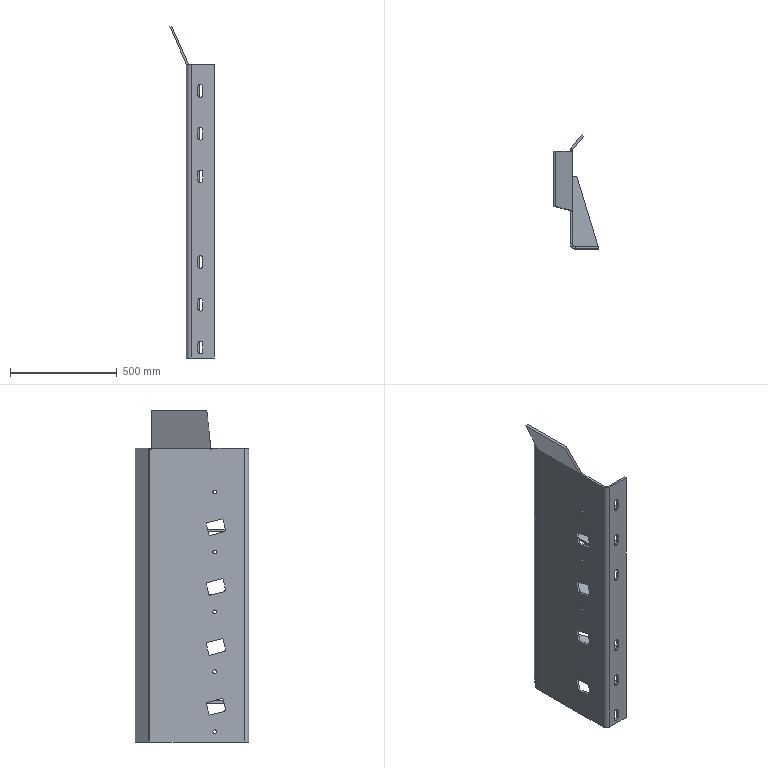Part | STEP file | Edge plate 4_Default<As machined> | 6 solids | 127 faces | box 207.636 x 532.359 x 1552 mm | volume 10466658 mm3 | plane 89 | cylinder 37 | spline 1 | commonest cylinder face diameters 24 x20 17 x10 30 x4 4 x2 44 x1